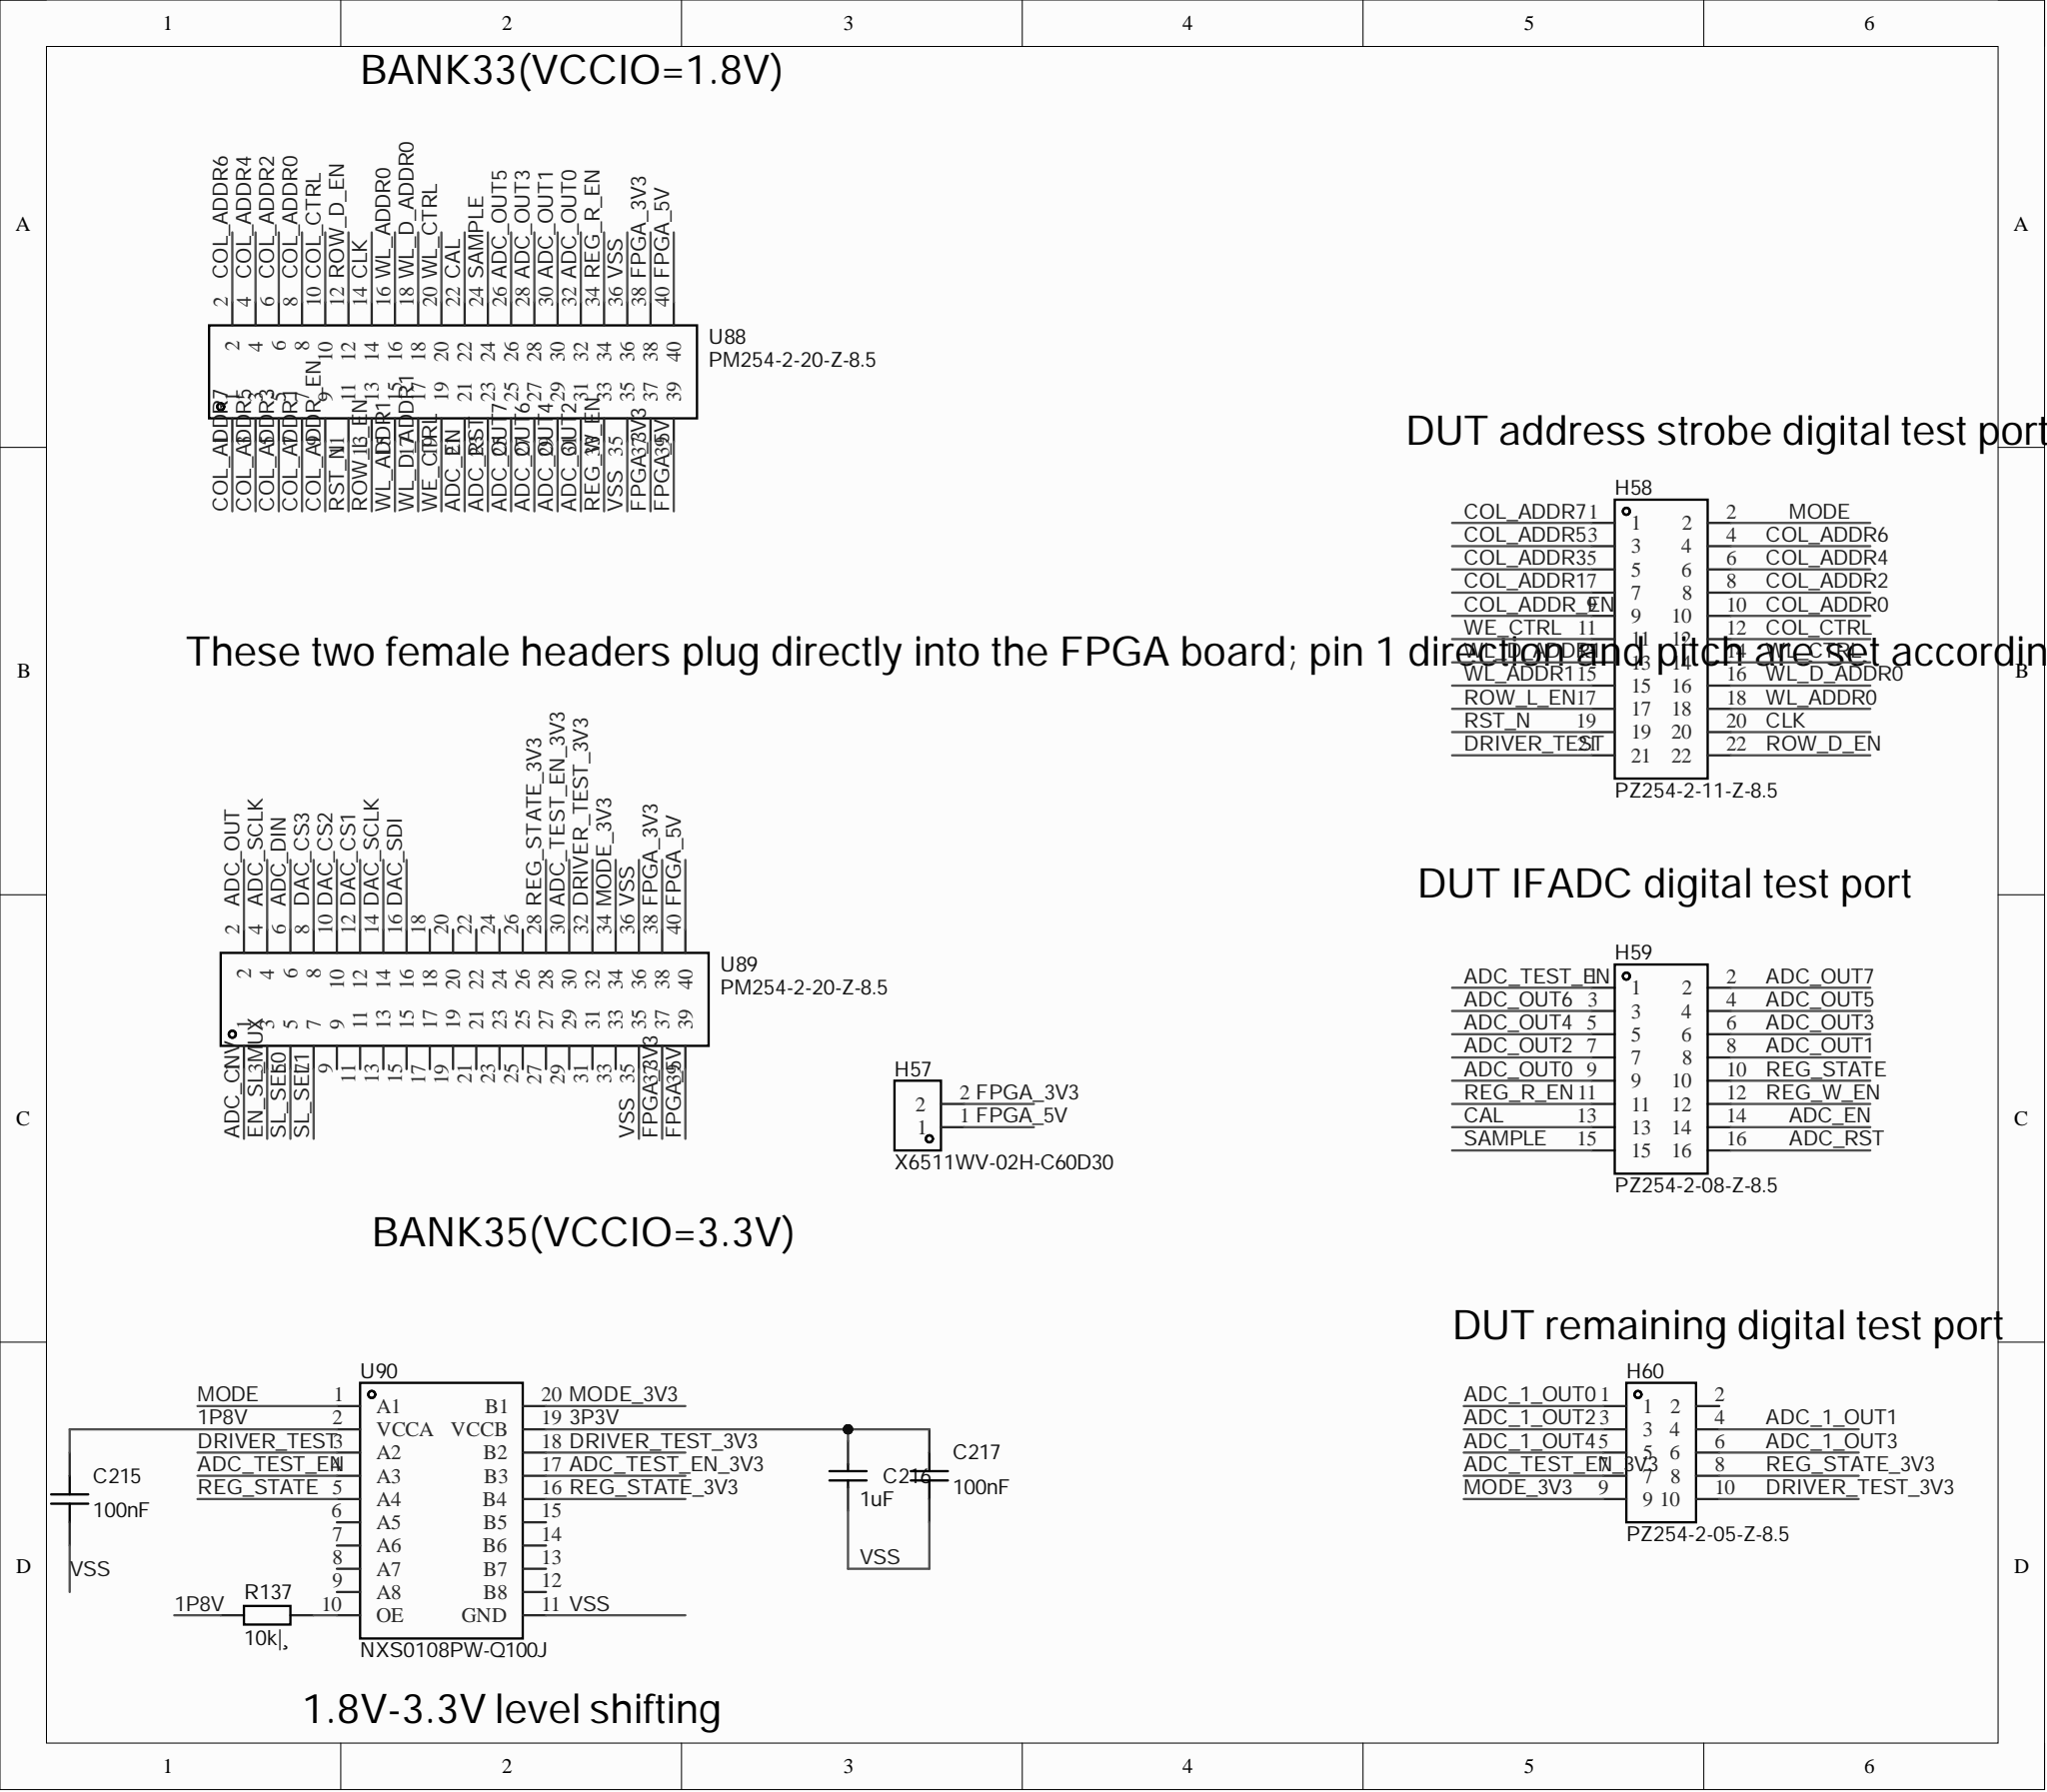Circuit board | Altium Designer | 201 parts | 197 nets | one sheet of the schematic
Parts on this sheet (reference | value | footprint):
C215 | 100nF | C0402
C216 | 1uF | C0603
C217 | 100nF | C0402
H57 | X6511WV-02H-C60D30 | HDR-TH_2P-P2.54-V-M
H58 | PZ254-2-11-Z-8.5 | HDR-TH_22P-P2.54-V-M-R2-C11-S2.54
H59 | PZ254-2-08-Z-8.5 | HDR-TH_16P-P2.54-V-M-R2-C8-S2.54
H60 | PZ254-2-05-Z-8.5 | HDR-TH_10P-P2.54-V-M-R2-C5-S2.54
R137 | 10k|¸ | R0603
U88 | PM254-2-20-Z-8.5 | HDR-TH_40P-P2.54-V-F-R2-C20-S2.54
U89 | PM254-2-20-Z-8.5 | HDR-TH_40P-P2.54-V-F-R2-C20-S2.54
U90 | NXS0108PW-Q100J | TSSOP-20_L6.5-W4.4-P0.65-LS6.4-BL
Nets of these parts (net: part-pin ...):
WL_D_ADDR1: H58-13 U88-17
WL_D_ADDR0: H58-16 U88-18
WL_CTRL: H58-14 U88-20
WL_ADDR1: H58-15 U88-15
WL_ADDR0: H58-18 U88-16
WE_CTRL: H58-11 U88-19
VSS: C215-1 C216-1 C217-1 U90-11 U88-35 U88-36 U89-35 U89-36
SL_SEL1: U89-7
SL_SEL0: U89-5
SAMPLE: H59-15 U88-24
RST_N: H58-19 U88-11
ROW_L_EN: H58-17 U88-13
ROW_D_EN: H58-22 U88-12
REG_W_EN: H59-12 U88-33
REG_STATE_3V3: H60-8 U90-16 U89-28
REG_STATE: H59-10 U90-5
REG_R_EN: H59-11 U88-34
NetR137_2: R137-2 U90-10
MODE_3V3: H60-9 U90-20 U89-34
MODE: U90-1 H58-2
FPGA_5V: H57-1 U88-39 U88-40 U89-39 U89-40
FPGA_3V3: H57-2 U88-37 U88-38 U89-37 U89-38
EN_SL_MUX: U89-3
DRIVER_TEST_3V3: H60-10 U90-18 U89-32
DRIVER_TEST: U90-3 H58-21
DAC_SDI: U89-16
DAC_SCLK: U89-14
DAC_CS3: U89-8
DAC_CS2: U89-10
DAC_CS1: U89-12
COL_CTRL: H58-12 U88-10
COL_ADDR_EN: H58-9 U88-9
COL_ADDR7: H58-1 U88-1
COL_ADDR6: H58-4 U88-2
COL_ADDR5: H58-3 U88-3
COL_ADDR4: H58-6 U88-4
COL_ADDR3: H58-5 U88-5
COL_ADDR2: H58-8 U88-6
COL_ADDR1: H58-7 U88-7
COL_ADDR0: H58-10 U88-8
CLK: H58-20 U88-14
CAL: H59-13 U88-22
ADC_TEST_EN_3V3: H60-7 U90-17 U89-30
ADC_TEST_EN: H59-1 U90-4
ADC_SCLK: U89-4
ADC_RST: H59-16 U88-23
ADC_OUT7: H59-2 U88-25
ADC_OUT6: H59-3 U88-27
ADC_OUT5: H59-4 U88-26
ADC_OUT4: H59-5 U88-29
ADC_OUT3: H59-6 U88-28
ADC_OUT2: H59-7 U88-31
ADC_OUT1: H59-8 U88-30
ADC_OUT0: H59-9 U88-32
ADC_OUT: U89-2
ADC_EN: H59-14 U88-21
ADC_DIN: U89-6
ADC_CNV: U89-1
ADC_1_OUT4: H60-5
ADC_1_OUT3: H60-6
ADC_1_OUT2: H60-3
ADC_1_OUT1: H60-4
ADC_1_OUT0: H60-1
3P3V: C216-2 C217-2 U90-19
1P8V: C215-2 R137-1 U90-2